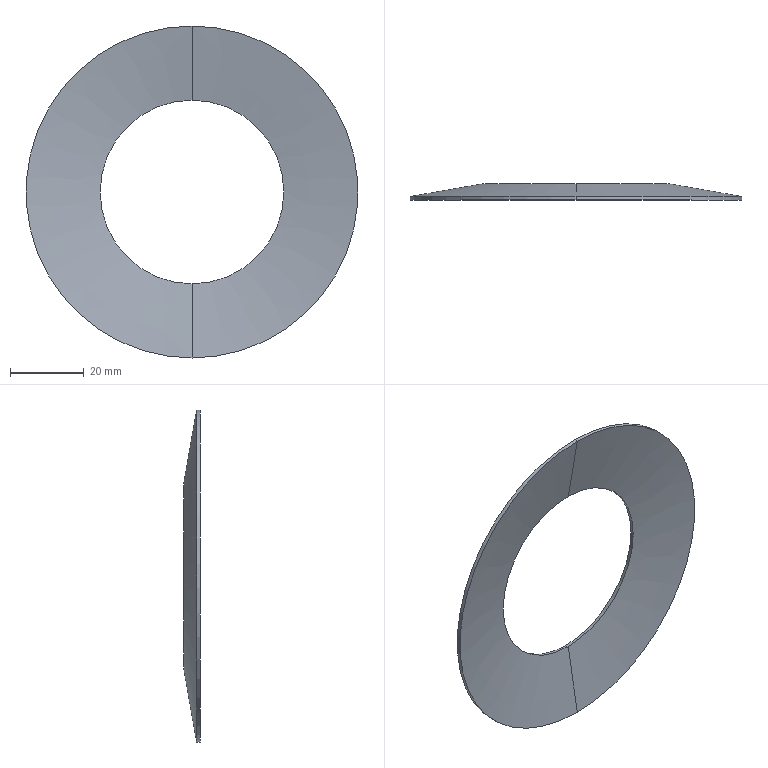Part | STEP file | Disc spring | 1 solid | 8 faces | box 90 x 4.485 x 90 mm | volume 4464 mm3 | cone 6 | cylinder 2 | commonest cylinder face diameters 90 x2
STEP:
#1=CARTESIAN_POINT('',(0.,52.647,-24.913));
#2=VERTEX_POINT('',#1);
#3=CARTESIAN_POINT('',(0.,52.647,24.913));
#4=VERTEX_POINT('',#3);
#5=CARTESIAN_POINT('',(0.,52.647,0.));
#6=DIRECTION('',(0.,1.,0.));
#7=DIRECTION('',(0.,0.,1.));
#8=AXIS2_PLACEMENT_3D('',#5,#6,#7);
#9=CIRCLE('',#8,24.913);
#10=EDGE_CURVE('',#2,#4,#9,.T.);
#11=ORIENTED_EDGE('',*,*,#10,.F.);
#12=CARTESIAN_POINT('',(0.,53.632,-25.087));
#13=VERTEX_POINT('',#12);
#14=CARTESIAN_POINT('',(0.,53.139,-25.));
#15=DIRECTION('',(0.,0.9847,-0.1743));
#16=VECTOR('',#15,1000.);
#17=LINE('',#14,#16);
#18=EDGE_CURVE('',#2,#13,#17,.T.);
#19=ORIENTED_EDGE('',*,*,#18,.T.);
#20=CARTESIAN_POINT('',(0.,53.632,25.087));
#21=VERTEX_POINT('',#20);
#22=CARTESIAN_POINT('',(0.,53.632,0.));
#23=DIRECTION('',(0.,1.,0.));
#24=DIRECTION('',(0.,0.,1.));
#25=AXIS2_PLACEMENT_3D('',#22,#23,#24);
#26=CIRCLE('',#25,25.087);
#27=EDGE_CURVE('',#13,#21,#26,.T.);
#28=ORIENTED_EDGE('',*,*,#27,.T.);
#29=CARTESIAN_POINT('',(0.,53.139,25.));
#30=DIRECTION('',(0.,0.9847,0.1743));
#31=VECTOR('',#30,1000.);
#32=LINE('',#29,#31);
#33=EDGE_CURVE('',#4,#21,#32,.T.);
#34=ORIENTED_EDGE('',*,*,#33,.F.);
#35=EDGE_LOOP('',(#11,#19,#28,#34));
#36=FACE_OUTER_BOUND('',#35,.T.);
#37=CARTESIAN_POINT('',(0.,53.139,0.));
#38=DIRECTION('',(0.,1.,0.));
#39=DIRECTION('',(0.,0.,1.));
#40=AXIS2_PLACEMENT_3D('',#37,#38,#39);
#41=CONICAL_SURFACE('',#40,25.,0.1752);
#42=ADVANCED_FACE('',(#36),#41,.F.);
#43=ORIENTED_EDGE('',*,*,#10,.T.);
#44=CARTESIAN_POINT('',(0.,49.147,45.));
#45=VERTEX_POINT('',#44);
#46=CARTESIAN_POINT('',(0.,49.147,45.));
#47=DIRECTION('',(0.,-0.1717,0.9852));
#48=VECTOR('',#47,1000.);
#49=LINE('',#46,#48);
#50=EDGE_CURVE('',#4,#45,#49,.T.);
#51=ORIENTED_EDGE('',*,*,#50,.T.);
#52=CARTESIAN_POINT('',(0.,49.147,-45.));
#53=VERTEX_POINT('',#52);
#54=CARTESIAN_POINT('',(0.,49.147,0.));
#55=DIRECTION('',(0.,1.,0.));
#56=DIRECTION('',(0.,0.,1.));
#57=AXIS2_PLACEMENT_3D('',#54,#55,#56);
#58=CIRCLE('',#57,45.);
#59=EDGE_CURVE('',#53,#45,#58,.T.);
#60=ORIENTED_EDGE('',*,*,#59,.F.);
#61=CARTESIAN_POINT('',(0.,49.147,-45.));
#62=DIRECTION('',(0.,-0.1717,-0.9852));
#63=VECTOR('',#62,1000.);
#64=LINE('',#61,#63);
#65=EDGE_CURVE('',#2,#53,#64,.T.);
#66=ORIENTED_EDGE('',*,*,#65,.F.);
#67=EDGE_LOOP('',(#43,#51,#60,#66));
#68=FACE_OUTER_BOUND('',#67,.T.);
#69=CARTESIAN_POINT('',(0.,49.147,0.));
#70=DIRECTION('',(0.,-1.,0.));
#71=DIRECTION('',(0.,0.,-1.));
#72=AXIS2_PLACEMENT_3D('',#69,#70,#71);
#73=CONICAL_SURFACE('',#72,45.,1.398);
#74=ADVANCED_FACE('',(#68),#73,.F.);
#75=CARTESIAN_POINT('',(0.,49.147,0.));
#76=DIRECTION('',(0.,1.,0.));
#77=DIRECTION('',(0.,0.,1.));
#78=AXIS2_PLACEMENT_3D('',#75,#76,#77);
#79=CIRCLE('',#78,45.);
#80=EDGE_CURVE('',#45,#53,#79,.T.);
#81=ORIENTED_EDGE('',*,*,#80,.T.);
#82=CARTESIAN_POINT('',(0.,50.162,-45.));
#83=VERTEX_POINT('',#82);
#84=CARTESIAN_POINT('',(0.,258.802,-45.));
#85=DIRECTION('',(0.,1.,0.));
#86=VECTOR('',#85,1000.);
#87=LINE('',#84,#86);
#88=EDGE_CURVE('',#53,#83,#87,.T.);
#89=ORIENTED_EDGE('',*,*,#88,.T.);
#90=CARTESIAN_POINT('',(0.,50.162,45.));
#91=VERTEX_POINT('',#90);
#92=CARTESIAN_POINT('',(0.,50.162,0.));
#93=DIRECTION('',(0.,1.,0.));
#94=DIRECTION('',(0.,0.,1.));
#95=AXIS2_PLACEMENT_3D('',#92,#93,#94);
#96=CIRCLE('',#95,45.);
#97=EDGE_CURVE('',#91,#83,#96,.T.);
#98=ORIENTED_EDGE('',*,*,#97,.F.);
#99=CARTESIAN_POINT('',(0.,258.802,45.));
#100=DIRECTION('',(0.,1.,0.));
#101=VECTOR('',#100,1000.);
#102=LINE('',#99,#101);
#103=EDGE_CURVE('',#45,#91,#102,.T.);
#104=ORIENTED_EDGE('',*,*,#103,.F.);
#105=EDGE_LOOP('',(#81,#89,#98,#104));
#106=FACE_OUTER_BOUND('',#105,.T.);
#107=CARTESIAN_POINT('',(0.,258.802,0.));
#108=DIRECTION('',(0.,1.,0.));
#109=DIRECTION('',(0.,0.,1.));
#110=AXIS2_PLACEMENT_3D('',#107,#108,#109);
#111=CYLINDRICAL_SURFACE('',#110,45.);
#112=ADVANCED_FACE('',(#106),#111,.T.);
#113=CARTESIAN_POINT('',(0.,53.632,0.));
#114=DIRECTION('',(0.,1.,0.));
#115=DIRECTION('',(0.,0.,1.));
#116=AXIS2_PLACEMENT_3D('',#113,#114,#115);
#117=CIRCLE('',#116,25.087);
#118=EDGE_CURVE('',#21,#13,#117,.T.);
#119=ORIENTED_EDGE('',*,*,#118,.F.);
#120=CARTESIAN_POINT('',(0.,53.632,25.087));
#121=DIRECTION('',(0.,-0.1717,0.9852));
#122=VECTOR('',#121,1000.);
#123=LINE('',#120,#122);
#124=EDGE_CURVE('',#21,#91,#123,.T.);
#125=ORIENTED_EDGE('',*,*,#124,.T.);
#126=ORIENTED_EDGE('',*,*,#97,.T.);
#127=CARTESIAN_POINT('',(0.,53.632,-25.087));
#128=DIRECTION('',(0.,-0.1717,-0.9852));
#129=VECTOR('',#128,1000.);
#130=LINE('',#127,#129);
#131=EDGE_CURVE('',#13,#83,#130,.T.);
#132=ORIENTED_EDGE('',*,*,#131,.F.);
#133=EDGE_LOOP('',(#119,#125,#126,#132));
#134=FACE_OUTER_BOUND('',#133,.T.);
#135=CARTESIAN_POINT('',(0.,53.632,0.));
#136=DIRECTION('',(0.,-1.,0.));
#137=DIRECTION('',(0.,0.,-1.));
#138=AXIS2_PLACEMENT_3D('',#135,#136,#137);
#139=CONICAL_SURFACE('',#138,25.087,1.398);
#140=ADVANCED_FACE('',(#134),#139,.T.);
#141=ORIENTED_EDGE('',*,*,#124,.F.);
#142=ORIENTED_EDGE('',*,*,#27,.F.);
#143=ORIENTED_EDGE('',*,*,#131,.T.);
#144=CARTESIAN_POINT('',(0.,50.162,0.));
#145=DIRECTION('',(0.,1.,0.));
#146=DIRECTION('',(0.,0.,1.));
#147=AXIS2_PLACEMENT_3D('',#144,#145,#146);
#148=CIRCLE('',#147,45.);
#149=EDGE_CURVE('',#83,#91,#148,.T.);
#150=ORIENTED_EDGE('',*,*,#149,.T.);
#151=EDGE_LOOP('',(#141,#142,#143,#150));
#152=FACE_OUTER_BOUND('',#151,.T.);
#153=CARTESIAN_POINT('',(0.,53.632,0.));
#154=DIRECTION('',(0.,-1.,0.));
#155=DIRECTION('',(0.,0.,-1.));
#156=AXIS2_PLACEMENT_3D('',#153,#154,#155);
#157=CONICAL_SURFACE('',#156,25.087,1.398);
#158=ADVANCED_FACE('',(#152),#157,.T.);
#159=ORIENTED_EDGE('',*,*,#88,.F.);
#160=ORIENTED_EDGE('',*,*,#59,.T.);
#161=ORIENTED_EDGE('',*,*,#103,.T.);
#162=ORIENTED_EDGE('',*,*,#149,.F.);
#163=EDGE_LOOP('',(#159,#160,#161,#162));
#164=FACE_OUTER_BOUND('',#163,.T.);
#165=CARTESIAN_POINT('',(0.,258.802,0.));
#166=DIRECTION('',(0.,1.,0.));
#167=DIRECTION('',(0.,0.,1.));
#168=AXIS2_PLACEMENT_3D('',#165,#166,#167);
#169=CYLINDRICAL_SURFACE('',#168,45.);
#170=ADVANCED_FACE('',(#164),#169,.T.);
#171=ORIENTED_EDGE('',*,*,#50,.F.);
#172=CARTESIAN_POINT('',(0.,52.647,0.));
#173=DIRECTION('',(0.,1.,0.));
#174=DIRECTION('',(0.,0.,1.));
#175=AXIS2_PLACEMENT_3D('',#172,#173,#174);
#176=CIRCLE('',#175,24.913);
#177=EDGE_CURVE('',#4,#2,#176,.T.);
#178=ORIENTED_EDGE('',*,*,#177,.T.);
#179=ORIENTED_EDGE('',*,*,#65,.T.);
#180=ORIENTED_EDGE('',*,*,#80,.F.);
#181=EDGE_LOOP('',(#171,#178,#179,#180));
#182=FACE_OUTER_BOUND('',#181,.T.);
#183=CARTESIAN_POINT('',(0.,49.147,0.));
#184=DIRECTION('',(0.,-1.,0.));
#185=DIRECTION('',(0.,0.,-1.));
#186=AXIS2_PLACEMENT_3D('',#183,#184,#185);
#187=CONICAL_SURFACE('',#186,45.,1.398);
#188=ADVANCED_FACE('',(#182),#187,.F.);
#189=ORIENTED_EDGE('',*,*,#18,.F.);
#190=ORIENTED_EDGE('',*,*,#177,.F.);
#191=ORIENTED_EDGE('',*,*,#33,.T.);
#192=ORIENTED_EDGE('',*,*,#118,.T.);
#193=EDGE_LOOP('',(#189,#190,#191,#192));
#194=FACE_OUTER_BOUND('',#193,.T.);
#195=CARTESIAN_POINT('',(0.,53.139,0.));
#196=DIRECTION('',(0.,1.,0.));
#197=DIRECTION('',(0.,0.,1.));
#198=AXIS2_PLACEMENT_3D('',#195,#196,#197);
#199=CONICAL_SURFACE('',#198,25.,0.1752);
#200=ADVANCED_FACE('',(#194),#199,.F.);
#201=CLOSED_SHELL('',(#42,#74,#112,#140,#158,#170,#188,#200));
#202=MANIFOLD_SOLID_BREP('',#201);
#203=CARTESIAN_POINT('',(0.,0.,0.));
#204=DIRECTION('',(0.,0.,1.));
#205=DIRECTION('',(1.,0.,0.));
#206=AXIS2_PLACEMENT_3D('',#203,#204,#205);
#207=(LENGTH_UNIT()NAMED_UNIT(*)SI_UNIT(.MILLI.,.METRE.));
#208=UNCERTAINTY_MEASURE_WITH_UNIT(LENGTH_MEASURE(0.00001),#207,'','');
#209=(NAMED_UNIT(*)PLANE_ANGLE_UNIT()SI_UNIT($,.RADIAN.));
#210=(NAMED_UNIT(*)SI_UNIT($,.STERADIAN.)SOLID_ANGLE_UNIT());
#211=(GEOMETRIC_REPRESENTATION_CONTEXT(3)GLOBAL_UNCERTAINTY_ASSIGNED_CONTEXT((#208))GLOBAL_UNIT_ASSIGNED_CONTEXT((#207,#209,#210))REPRESENTATION_CONTEXT('',''));
#212=ADVANCED_BREP_SHAPE_REPRESENTATION('',(#202,#206),#211);